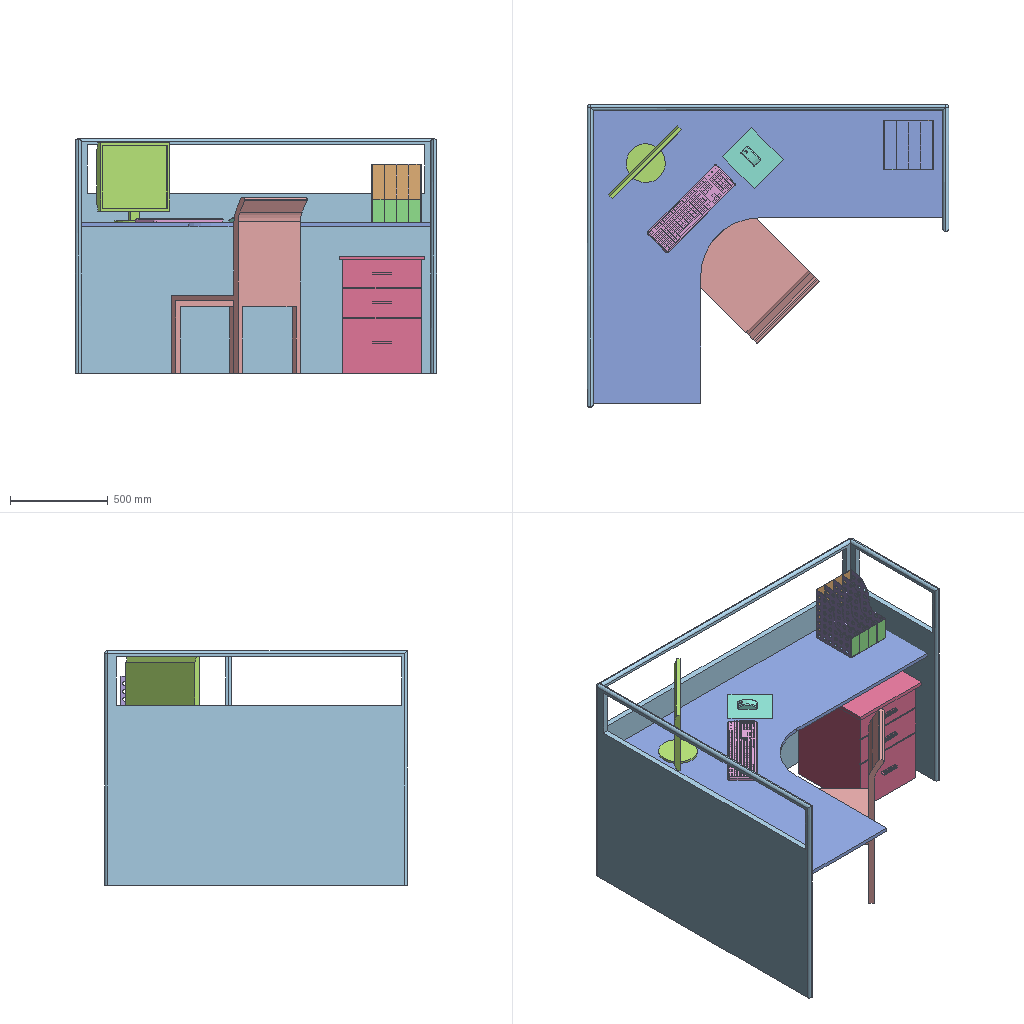Assembly | SolidWorks | 11 different items | 15 placed | box 1850 x 1550 x 1200 mm
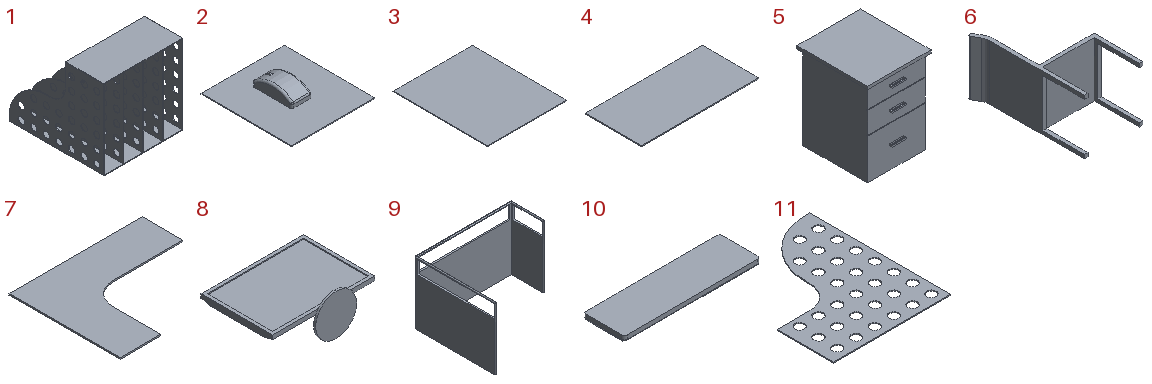Parts list (item | name | quantity | parent item | size | volume | features):
1 | (subassembly) | x1 | - | 252 x 300 x 254 mm | 627356 mm3 | features ReferencePattern 4, LocalLPattern 1, MateUpdatePoint 1
2 | - | x1 | - | 210 x 230 x 32 mm | 215921 mm3 | features ICE 4, Fillet 2, Extrusion 1
3 | - | x1 | in 1 | 250 x 300 x 2 mm | 150000 mm3 | features Extrusion 1
4 | - | x1 | in 1 | 250 x 120 x 2 mm | 60000 mm3 | features Extrusion 1
5 | - | x1 | - | 440 x 490 x 600 mm | 108712401 mm3 | features ICE 7, Extrusion 1
6 | - | x1 | - | 529.703 x 900 x 450 mm | 15410155 mm3 | features Extrusion 1, ICE 1
7 | - | x1 | - | 1800 x 1500 x 20 mm | 30636283 mm3 | features Extrusion 1
8 | - | x1 | - | 500 x 410 x 200 mm | 4616159 mm3 | features ICE 4, Extrusion 1
9 | - | x1 | - | 1850 x 1550 x 1200 mm | 114783805 mm3 | features ICE 3, Extrusion 1, Fillet 1
10 | - | x1 | - | 500 x 150 x 24 mm | 1615736 mm3 | features ICE 6, Fillet 2, Extrusion 1
11 | - | x5 | in 1 | 250 x 300 x 2 mm | 83471 mm3 | features Extrusion 1, ICE 1
Mates (type | each side: item.copy, entity, surface, feature):
In the top assembly
Coincident | 7.1 face plane Boss-Extrude1 | 8.1 face plane Boss-Extrude4
DistanceDim | 6.1 face plane Boss-Extrude1 | 8.1 face plane Cut-Extrude1
Coincident | 6.1 face plane Boss-Extrude1 | 8.1 face plane Boss-Extrude1
Coincident | 7.1 face plane Boss-Extrude1 | 10.1 face plane Boss-Extrude1
DistanceDim | 10.1 face plane Boss-Extrude1 | 8.1 face plane Cut-Extrude1
Coincident | 8.1 face plane Boss-Extrude1 | 10.1 face plane Boss-Extrude1
Coincident | 7.1 face plane Boss-Extrude1 | 2.1 face plane Boss-Extrude3
DistanceDim | 2.1 face plane Boss-Extrude3 | 10.1 face plane Boss-Extrude1
Coincident | 10.1 face plane Boss-Extrude1 | 2.1 face plane Boss-Extrude3
Coincident | 7.1 face plane Boss-Extrude1 | 4.1 face plane Boss-Extrude1
Coincident | 7.1 face plane Boss-Extrude1 | 9.1 face plane Boss-Extrude2 | 2 times
DistanceDim | 7.1 face plane Boss-Extrude1 | 9.1 face plane Boss-Extrude2
DistanceDim | 5.1 face plane Boss-Extrude1 | 9.1 face plane Boss-Extrude2 | 2 times
Coincident | 5.1 face plane Boss-Extrude1 | 9.1 face plane Boss-Extrude2
Coincident | 6.1 face plane Boss-Extrude1 | 5.1 face plane Boss-Extrude1
DistanceDim | 11.1 face plane Boss-Extrude1 | 9.1 face plane Boss-Extrude2
DistanceDim | 3.1 face plane Boss-Extrude1 | 9.1 face plane Boss-Extrude2
DistanceDim | 8.1 edge | 9.1 face plane Boss-Extrude2 | 2 times
PlanarAngleDim | 8.1 face plane Cut-Extrude1 | 9.1 face plane Boss-Extrude2
In subassembly 1
Coincident | 3.2 face plane Boss-Extrude1 | 11.2 face plane Boss-Extrude1 | 3 times
Coincident | 11.3 face plane Boss-Extrude1 | 4.2 face plane Boss-Extrude1 | 2 times
Coincident | 11.4 face plane Boss-Extrude1 | 4.2 face plane Boss-Extrude1